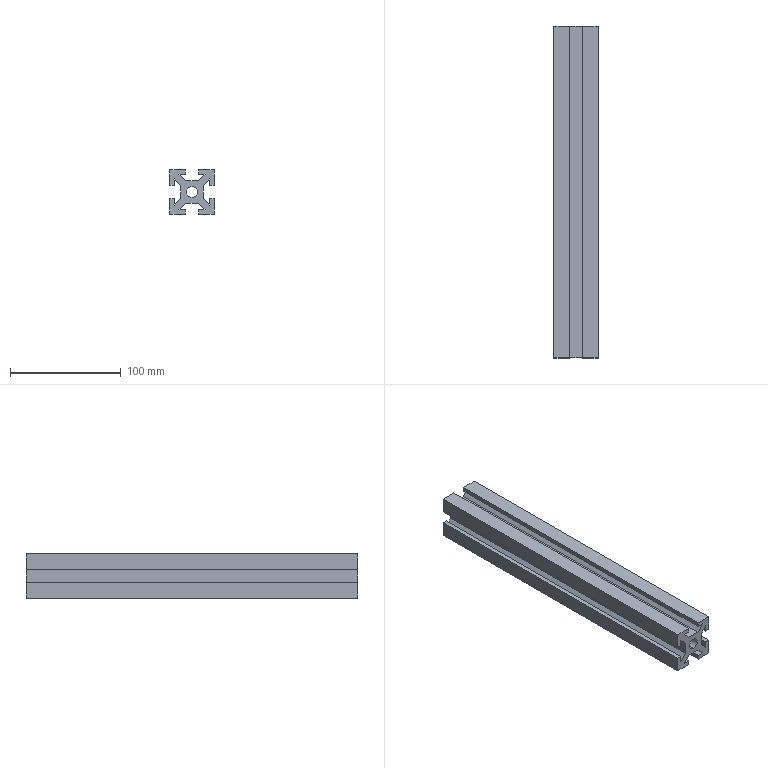Part | SolidWorks | features Extrusion 1 | 1 solid | 40 faces | box 40 x 300 x 40 mm | volume 272732 mm3 | plane 38 | cylinder 2 | commonest cylinder face diameters 10 x2
STEP:
#1=CARTESIAN_POINT('',(0.,300.,-5.));
#2=VERTEX_POINT('',#1);
#3=CARTESIAN_POINT('',(0.,300.,5.));
#4=VERTEX_POINT('',#3);
#5=CARTESIAN_POINT('',(0.,300.,0.));
#6=DIRECTION('',(0.,1.,0.));
#7=DIRECTION('',(0.,0.,1.));
#8=AXIS2_PLACEMENT_3D('',#5,#6,#7);
#9=CIRCLE('',#8,5.);
#10=EDGE_CURVE('',#2,#4,#9,.T.);
#11=ORIENTED_EDGE('',*,*,#10,.T.);
#12=CARTESIAN_POINT('',(0.,0.,5.));
#13=VERTEX_POINT('',#12);
#14=CARTESIAN_POINT('',(0.,300.,5.));
#15=DIRECTION('',(0.,-1.,0.));
#16=VECTOR('',#15,1000.);
#17=LINE('',#14,#16);
#18=EDGE_CURVE('',#4,#13,#17,.T.);
#19=ORIENTED_EDGE('',*,*,#18,.T.);
#20=CARTESIAN_POINT('',(0.,0.,-5.));
#21=VERTEX_POINT('',#20);
#22=CARTESIAN_POINT('',(0.,0.,0.));
#23=DIRECTION('',(0.,1.,0.));
#24=DIRECTION('',(0.,0.,1.));
#25=AXIS2_PLACEMENT_3D('',#22,#23,#24);
#26=CIRCLE('',#25,5.);
#27=EDGE_CURVE('',#21,#13,#26,.T.);
#28=ORIENTED_EDGE('',*,*,#27,.F.);
#29=CARTESIAN_POINT('',(0.,300.,-5.));
#30=DIRECTION('',(0.,-1.,0.));
#31=VECTOR('',#30,1000.);
#32=LINE('',#29,#31);
#33=EDGE_CURVE('',#2,#21,#32,.T.);
#34=ORIENTED_EDGE('',*,*,#33,.F.);
#35=EDGE_LOOP('',(#11,#19,#28,#34));
#36=FACE_OUTER_BOUND('',#35,.T.);
#37=CARTESIAN_POINT('',(0.,300.,0.));
#38=DIRECTION('',(0.,-1.,0.));
#39=DIRECTION('',(0.,0.,-1.));
#40=AXIS2_PLACEMENT_3D('',#37,#38,#39);
#41=CYLINDRICAL_SURFACE('',#40,5.);
#42=ADVANCED_FACE('',(#36),#41,.F.);
#43=CARTESIAN_POINT('',(6.,300.,20.));
#44=VERTEX_POINT('',#43);
#45=CARTESIAN_POINT('',(20.,300.,20.));
#46=VERTEX_POINT('',#45);
#47=CARTESIAN_POINT('',(6.,300.,20.));
#48=DIRECTION('',(1.,0.,0.));
#49=VECTOR('',#48,1000.);
#50=LINE('',#47,#49);
#51=EDGE_CURVE('',#44,#46,#50,.T.);
#52=ORIENTED_EDGE('',*,*,#51,.T.);
#53=CARTESIAN_POINT('',(20.,300.,6.));
#54=VERTEX_POINT('',#53);
#55=CARTESIAN_POINT('',(20.,300.,6.));
#56=DIRECTION('',(0.,0.,-1.));
#57=VECTOR('',#56,1000.);
#58=LINE('',#55,#57);
#59=EDGE_CURVE('',#46,#54,#58,.T.);
#60=ORIENTED_EDGE('',*,*,#59,.T.);
#61=CARTESIAN_POINT('',(16.,300.,6.));
#62=VERTEX_POINT('',#61);
#63=CARTESIAN_POINT('',(16.,300.,6.));
#64=DIRECTION('',(-1.,0.,0.));
#65=VECTOR('',#64,1000.);
#66=LINE('',#63,#65);
#67=EDGE_CURVE('',#54,#62,#66,.T.);
#68=ORIENTED_EDGE('',*,*,#67,.T.);
#69=CARTESIAN_POINT('',(16.,300.,11.757));
#70=VERTEX_POINT('',#69);
#71=CARTESIAN_POINT('',(16.,300.,11.757));
#72=DIRECTION('',(0.,0.,1.));
#73=VECTOR('',#72,1000.);
#74=LINE('',#71,#73);
#75=EDGE_CURVE('',#62,#70,#74,.T.);
#76=ORIENTED_EDGE('',*,*,#75,.T.);
#77=CARTESIAN_POINT('',(10.,300.,5.757));
#78=VERTEX_POINT('',#77);
#79=CARTESIAN_POINT('',(10.,300.,5.757));
#80=DIRECTION('',(-0.7071,0.,-0.7071));
#81=VECTOR('',#80,1000.);
#82=LINE('',#79,#81);
#83=EDGE_CURVE('',#70,#78,#82,.T.);
#84=ORIENTED_EDGE('',*,*,#83,.T.);
#85=CARTESIAN_POINT('',(10.,300.,-5.757));
#86=VERTEX_POINT('',#85);
#87=CARTESIAN_POINT('',(10.,300.,5.757));
#88=DIRECTION('',(0.,0.,-1.));
#89=VECTOR('',#88,1000.);
#90=LINE('',#87,#89);
#91=EDGE_CURVE('',#78,#86,#90,.T.);
#92=ORIENTED_EDGE('',*,*,#91,.T.);
#93=CARTESIAN_POINT('',(16.,300.,-11.757));
#94=VERTEX_POINT('',#93);
#95=CARTESIAN_POINT('',(16.,300.,-11.757));
#96=DIRECTION('',(0.7071,0.,-0.7071));
#97=VECTOR('',#96,1000.);
#98=LINE('',#95,#97);
#99=EDGE_CURVE('',#86,#94,#98,.T.);
#100=ORIENTED_EDGE('',*,*,#99,.T.);
#101=CARTESIAN_POINT('',(16.,300.,-6.));
#102=VERTEX_POINT('',#101);
#103=CARTESIAN_POINT('',(16.,300.,-6.));
#104=DIRECTION('',(0.,0.,1.));
#105=VECTOR('',#104,1000.);
#106=LINE('',#103,#105);
#107=EDGE_CURVE('',#94,#102,#106,.T.);
#108=ORIENTED_EDGE('',*,*,#107,.T.);
#109=CARTESIAN_POINT('',(20.,300.,-6.));
#110=VERTEX_POINT('',#109);
#111=CARTESIAN_POINT('',(20.,300.,-6.));
#112=DIRECTION('',(1.,0.,0.));
#113=VECTOR('',#112,1000.);
#114=LINE('',#111,#113);
#115=EDGE_CURVE('',#102,#110,#114,.T.);
#116=ORIENTED_EDGE('',*,*,#115,.T.);
#117=CARTESIAN_POINT('',(20.,300.,-20.));
#118=VERTEX_POINT('',#117);
#119=CARTESIAN_POINT('',(20.,300.,-20.));
#120=DIRECTION('',(0.,0.,-1.));
#121=VECTOR('',#120,1000.);
#122=LINE('',#119,#121);
#123=EDGE_CURVE('',#110,#118,#122,.T.);
#124=ORIENTED_EDGE('',*,*,#123,.T.);
#125=CARTESIAN_POINT('',(6.,300.,-20.));
#126=VERTEX_POINT('',#125);
#127=CARTESIAN_POINT('',(6.,300.,-20.));
#128=DIRECTION('',(-1.,0.,0.));
#129=VECTOR('',#128,1000.);
#130=LINE('',#127,#129);
#131=EDGE_CURVE('',#118,#126,#130,.T.);
#132=ORIENTED_EDGE('',*,*,#131,.T.);
#133=CARTESIAN_POINT('',(6.,300.,-16.));
#134=VERTEX_POINT('',#133);
#135=CARTESIAN_POINT('',(6.,300.,-16.));
#136=DIRECTION('',(0.,0.,1.));
#137=VECTOR('',#136,1000.);
#138=LINE('',#135,#137);
#139=EDGE_CURVE('',#126,#134,#138,.T.);
#140=ORIENTED_EDGE('',*,*,#139,.T.);
#141=CARTESIAN_POINT('',(11.757,300.,-16.));
#142=VERTEX_POINT('',#141);
#143=CARTESIAN_POINT('',(11.757,300.,-16.));
#144=DIRECTION('',(1.,0.,0.));
#145=VECTOR('',#144,1000.);
#146=LINE('',#143,#145);
#147=EDGE_CURVE('',#134,#142,#146,.T.);
#148=ORIENTED_EDGE('',*,*,#147,.T.);
#149=CARTESIAN_POINT('',(5.757,300.,-10.));
#150=VERTEX_POINT('',#149);
#151=CARTESIAN_POINT('',(5.757,300.,-10.));
#152=DIRECTION('',(-0.7071,0.,0.7071));
#153=VECTOR('',#152,1000.);
#154=LINE('',#151,#153);
#155=EDGE_CURVE('',#142,#150,#154,.T.);
#156=ORIENTED_EDGE('',*,*,#155,.T.);
#157=CARTESIAN_POINT('',(-5.757,300.,-10.));
#158=VERTEX_POINT('',#157);
#159=CARTESIAN_POINT('',(-5.757,300.,-10.));
#160=DIRECTION('',(-1.,0.,0.));
#161=VECTOR('',#160,1000.);
#162=LINE('',#159,#161);
#163=EDGE_CURVE('',#150,#158,#162,.T.);
#164=ORIENTED_EDGE('',*,*,#163,.T.);
#165=CARTESIAN_POINT('',(-11.757,300.,-16.));
#166=VERTEX_POINT('',#165);
#167=CARTESIAN_POINT('',(-11.757,300.,-16.));
#168=DIRECTION('',(-0.7071,0.,-0.7071));
#169=VECTOR('',#168,1000.);
#170=LINE('',#167,#169);
#171=EDGE_CURVE('',#158,#166,#170,.T.);
#172=ORIENTED_EDGE('',*,*,#171,.T.);
#173=CARTESIAN_POINT('',(-6.,300.,-16.));
#174=VERTEX_POINT('',#173);
#175=CARTESIAN_POINT('',(-6.,300.,-16.));
#176=DIRECTION('',(1.,0.,0.));
#177=VECTOR('',#176,1000.);
#178=LINE('',#175,#177);
#179=EDGE_CURVE('',#166,#174,#178,.T.);
#180=ORIENTED_EDGE('',*,*,#179,.T.);
#181=CARTESIAN_POINT('',(-6.,300.,-20.));
#182=VERTEX_POINT('',#181);
#183=CARTESIAN_POINT('',(-6.,300.,-20.));
#184=DIRECTION('',(0.,0.,-1.));
#185=VECTOR('',#184,1000.);
#186=LINE('',#183,#185);
#187=EDGE_CURVE('',#174,#182,#186,.T.);
#188=ORIENTED_EDGE('',*,*,#187,.T.);
#189=CARTESIAN_POINT('',(-20.,300.,-20.));
#190=VERTEX_POINT('',#189);
#191=CARTESIAN_POINT('',(-20.,300.,-20.));
#192=DIRECTION('',(-1.,0.,0.));
#193=VECTOR('',#192,1000.);
#194=LINE('',#191,#193);
#195=EDGE_CURVE('',#182,#190,#194,.T.);
#196=ORIENTED_EDGE('',*,*,#195,.T.);
#197=CARTESIAN_POINT('',(-20.,300.,-6.));
#198=VERTEX_POINT('',#197);
#199=CARTESIAN_POINT('',(-20.,300.,-20.));
#200=DIRECTION('',(0.,0.,1.));
#201=VECTOR('',#200,1000.);
#202=LINE('',#199,#201);
#203=EDGE_CURVE('',#190,#198,#202,.T.);
#204=ORIENTED_EDGE('',*,*,#203,.T.);
#205=CARTESIAN_POINT('',(-16.,300.,-6.));
#206=VERTEX_POINT('',#205);
#207=CARTESIAN_POINT('',(-16.,300.,-6.));
#208=DIRECTION('',(1.,0.,0.));
#209=VECTOR('',#208,1000.);
#210=LINE('',#207,#209);
#211=EDGE_CURVE('',#198,#206,#210,.T.);
#212=ORIENTED_EDGE('',*,*,#211,.T.);
#213=CARTESIAN_POINT('',(-16.,300.,-11.757));
#214=VERTEX_POINT('',#213);
#215=CARTESIAN_POINT('',(-16.,300.,-11.757));
#216=DIRECTION('',(0.,0.,-1.));
#217=VECTOR('',#216,1000.);
#218=LINE('',#215,#217);
#219=EDGE_CURVE('',#206,#214,#218,.T.);
#220=ORIENTED_EDGE('',*,*,#219,.T.);
#221=CARTESIAN_POINT('',(-10.,300.,-5.757));
#222=VERTEX_POINT('',#221);
#223=CARTESIAN_POINT('',(-10.,300.,-5.757));
#224=DIRECTION('',(0.7071,0.,0.7071));
#225=VECTOR('',#224,1000.);
#226=LINE('',#223,#225);
#227=EDGE_CURVE('',#214,#222,#226,.T.);
#228=ORIENTED_EDGE('',*,*,#227,.T.);
#229=CARTESIAN_POINT('',(-10.,300.,5.757));
#230=VERTEX_POINT('',#229);
#231=CARTESIAN_POINT('',(-10.,300.,5.757));
#232=DIRECTION('',(0.,0.,1.));
#233=VECTOR('',#232,1000.);
#234=LINE('',#231,#233);
#235=EDGE_CURVE('',#222,#230,#234,.T.);
#236=ORIENTED_EDGE('',*,*,#235,.T.);
#237=CARTESIAN_POINT('',(-16.,300.,11.757));
#238=VERTEX_POINT('',#237);
#239=CARTESIAN_POINT('',(-16.,300.,11.757));
#240=DIRECTION('',(-0.7071,0.,0.7071));
#241=VECTOR('',#240,1000.);
#242=LINE('',#239,#241);
#243=EDGE_CURVE('',#230,#238,#242,.T.);
#244=ORIENTED_EDGE('',*,*,#243,.T.);
#245=CARTESIAN_POINT('',(-16.,300.,6.));
#246=VERTEX_POINT('',#245);
#247=CARTESIAN_POINT('',(-16.,300.,6.));
#248=DIRECTION('',(0.,0.,-1.));
#249=VECTOR('',#248,1000.);
#250=LINE('',#247,#249);
#251=EDGE_CURVE('',#238,#246,#250,.T.);
#252=ORIENTED_EDGE('',*,*,#251,.T.);
#253=CARTESIAN_POINT('',(-20.,300.,6.));
#254=VERTEX_POINT('',#253);
#255=CARTESIAN_POINT('',(-20.,300.,6.));
#256=DIRECTION('',(-1.,0.,0.));
#257=VECTOR('',#256,1000.);
#258=LINE('',#255,#257);
#259=EDGE_CURVE('',#246,#254,#258,.T.);
#260=ORIENTED_EDGE('',*,*,#259,.T.);
#261=CARTESIAN_POINT('',(-20.,300.,20.));
#262=VERTEX_POINT('',#261);
#263=CARTESIAN_POINT('',(-20.,300.,6.));
#264=DIRECTION('',(0.,0.,1.));
#265=VECTOR('',#264,1000.);
#266=LINE('',#263,#265);
#267=EDGE_CURVE('',#254,#262,#266,.T.);
#268=ORIENTED_EDGE('',*,*,#267,.T.);
#269=CARTESIAN_POINT('',(-6.,300.,20.));
#270=VERTEX_POINT('',#269);
#271=CARTESIAN_POINT('',(-20.,300.,20.));
#272=DIRECTION('',(1.,0.,0.));
#273=VECTOR('',#272,1000.);
#274=LINE('',#271,#273);
#275=EDGE_CURVE('',#262,#270,#274,.T.);
#276=ORIENTED_EDGE('',*,*,#275,.T.);
#277=CARTESIAN_POINT('',(-6.,300.,16.));
#278=VERTEX_POINT('',#277);
#279=CARTESIAN_POINT('',(-6.,300.,16.));
#280=DIRECTION('',(0.,0.,-1.));
#281=VECTOR('',#280,1000.);
#282=LINE('',#279,#281);
#283=EDGE_CURVE('',#270,#278,#282,.T.);
#284=ORIENTED_EDGE('',*,*,#283,.T.);
#285=CARTESIAN_POINT('',(-11.757,300.,16.));
#286=VERTEX_POINT('',#285);
#287=CARTESIAN_POINT('',(-11.757,300.,16.));
#288=DIRECTION('',(-1.,0.,0.));
#289=VECTOR('',#288,1000.);
#290=LINE('',#287,#289);
#291=EDGE_CURVE('',#278,#286,#290,.T.);
#292=ORIENTED_EDGE('',*,*,#291,.T.);
#293=CARTESIAN_POINT('',(-5.757,300.,10.));
#294=VERTEX_POINT('',#293);
#295=CARTESIAN_POINT('',(-5.757,300.,10.));
#296=DIRECTION('',(0.7071,0.,-0.7071));
#297=VECTOR('',#296,1000.);
#298=LINE('',#295,#297);
#299=EDGE_CURVE('',#286,#294,#298,.T.);
#300=ORIENTED_EDGE('',*,*,#299,.T.);
#301=CARTESIAN_POINT('',(5.757,300.,10.));
#302=VERTEX_POINT('',#301);
#303=CARTESIAN_POINT('',(-5.757,300.,10.));
#304=DIRECTION('',(1.,0.,0.));
#305=VECTOR('',#304,1000.);
#306=LINE('',#303,#305);
#307=EDGE_CURVE('',#294,#302,#306,.T.);
#308=ORIENTED_EDGE('',*,*,#307,.T.);
#309=CARTESIAN_POINT('',(11.757,300.,16.));
#310=VERTEX_POINT('',#309);
#311=CARTESIAN_POINT('',(11.757,300.,16.));
#312=DIRECTION('',(0.7071,0.,0.7071));
#313=VECTOR('',#312,1000.);
#314=LINE('',#311,#313);
#315=EDGE_CURVE('',#302,#310,#314,.T.);
#316=ORIENTED_EDGE('',*,*,#315,.T.);
#317=CARTESIAN_POINT('',(6.,300.,16.));
#318=VERTEX_POINT('',#317);
#319=CARTESIAN_POINT('',(6.,300.,16.));
#320=DIRECTION('',(-1.,0.,0.));
#321=VECTOR('',#320,1000.);
#322=LINE('',#319,#321);
#323=EDGE_CURVE('',#310,#318,#322,.T.);
#324=ORIENTED_EDGE('',*,*,#323,.T.);
#325=CARTESIAN_POINT('',(6.,300.,20.));
#326=DIRECTION('',(0.,0.,1.));
#327=VECTOR('',#326,1000.);
#328=LINE('',#325,#327);
#329=EDGE_CURVE('',#318,#44,#328,.T.);
#330=ORIENTED_EDGE('',*,*,#329,.T.);
#331=EDGE_LOOP('',(#52,#60,#68,#76,#84,#92,#100,#108,#116,#124,#132,#140,#148,#156,#164,#172,#180,#188,#196,#204,#212,#220,#228,#236,#244,#252,#260,#268,#276,#284,#292,#300,#308,#316,#324,#330));
#332=FACE_OUTER_BOUND('',#331,.T.);
#333=ORIENTED_EDGE('',*,*,#10,.F.);
#334=CARTESIAN_POINT('',(0.,300.,0.));
#335=DIRECTION('',(0.,1.,0.));
#336=DIRECTION('',(0.,0.,1.));
#337=AXIS2_PLACEMENT_3D('',#334,#335,#336);
#338=CIRCLE('',#337,5.);
#339=EDGE_CURVE('',#4,#2,#338,.T.);
#340=ORIENTED_EDGE('',*,*,#339,.F.);
#341=EDGE_LOOP('',(#333,#340));
#342=FACE_BOUND('',#341,.T.);
#343=CARTESIAN_POINT('',(0.,300.,0.));
#344=DIRECTION('',(0.,-1.,0.));
#345=DIRECTION('',(0.,0.,-1.));
#346=AXIS2_PLACEMENT_3D('',#343,#344,#345);
#347=PLANE('',#346);
#348=ADVANCED_FACE('',(#332,#342),#347,.F.);
#349=CARTESIAN_POINT('',(6.,0.,20.));
#350=VERTEX_POINT('',#349);
#351=CARTESIAN_POINT('',(20.,0.,20.));
#352=VERTEX_POINT('',#351);
#353=CARTESIAN_POINT('',(6.,0.,20.));
#354=DIRECTION('',(1.,0.,0.));
#355=VECTOR('',#354,1000.);
#356=LINE('',#353,#355);
#357=EDGE_CURVE('',#350,#352,#356,.T.);
#358=ORIENTED_EDGE('',*,*,#357,.F.);
#359=CARTESIAN_POINT('',(6.,0.,16.));
#360=VERTEX_POINT('',#359);
#361=CARTESIAN_POINT('',(6.,0.,20.));
#362=DIRECTION('',(0.,0.,1.));
#363=VECTOR('',#362,1000.);
#364=LINE('',#361,#363);
#365=EDGE_CURVE('',#360,#350,#364,.T.);
#366=ORIENTED_EDGE('',*,*,#365,.F.);
#367=CARTESIAN_POINT('',(11.757,0.,16.));
#368=VERTEX_POINT('',#367);
#369=CARTESIAN_POINT('',(6.,0.,16.));
#370=DIRECTION('',(-1.,0.,0.));
#371=VECTOR('',#370,1000.);
#372=LINE('',#369,#371);
#373=EDGE_CURVE('',#368,#360,#372,.T.);
#374=ORIENTED_EDGE('',*,*,#373,.F.);
#375=CARTESIAN_POINT('',(5.757,0.,10.));
#376=VERTEX_POINT('',#375);
#377=CARTESIAN_POINT('',(11.757,0.,16.));
#378=DIRECTION('',(0.7071,0.,0.7071));
#379=VECTOR('',#378,1000.);
#380=LINE('',#377,#379);
#381=EDGE_CURVE('',#376,#368,#380,.T.);
#382=ORIENTED_EDGE('',*,*,#381,.F.);
#383=CARTESIAN_POINT('',(-5.757,0.,10.));
#384=VERTEX_POINT('',#383);
#385=CARTESIAN_POINT('',(-5.757,0.,10.));
#386=DIRECTION('',(1.,0.,0.));
#387=VECTOR('',#386,1000.);
#388=LINE('',#385,#387);
#389=EDGE_CURVE('',#384,#376,#388,.T.);
#390=ORIENTED_EDGE('',*,*,#389,.F.);
#391=CARTESIAN_POINT('',(-11.757,0.,16.));
#392=VERTEX_POINT('',#391);
#393=CARTESIAN_POINT('',(-5.757,0.,10.));
#394=DIRECTION('',(0.7071,0.,-0.7071));
#395=VECTOR('',#394,1000.);
#396=LINE('',#393,#395);
#397=EDGE_CURVE('',#392,#384,#396,.T.);
#398=ORIENTED_EDGE('',*,*,#397,.F.);
#399=CARTESIAN_POINT('',(-6.,0.,16.));
#400=VERTEX_POINT('',#399);
#401=CARTESIAN_POINT('',(-11.757,0.,16.));
#402=DIRECTION('',(-1.,0.,0.));
#403=VECTOR('',#402,1000.);
#404=LINE('',#401,#403);
#405=EDGE_CURVE('',#400,#392,#404,.T.);
#406=ORIENTED_EDGE('',*,*,#405,.F.);
#407=CARTESIAN_POINT('',(-6.,0.,20.));
#408=VERTEX_POINT('',#407);
#409=CARTESIAN_POINT('',(-6.,0.,16.));
#410=DIRECTION('',(0.,0.,-1.));
#411=VECTOR('',#410,1000.);
#412=LINE('',#409,#411);
#413=EDGE_CURVE('',#408,#400,#412,.T.);
#414=ORIENTED_EDGE('',*,*,#413,.F.);
#415=CARTESIAN_POINT('',(-20.,0.,20.));
#416=VERTEX_POINT('',#415);
#417=CARTESIAN_POINT('',(-20.,0.,20.));
#418=DIRECTION('',(1.,0.,0.));
#419=VECTOR('',#418,1000.);
#420=LINE('',#417,#419);
#421=EDGE_CURVE('',#416,#408,#420,.T.);
#422=ORIENTED_EDGE('',*,*,#421,.F.);
#423=CARTESIAN_POINT('',(-20.,0.,6.));
#424=VERTEX_POINT('',#423);
#425=CARTESIAN_POINT('',(-20.,0.,6.));
#426=DIRECTION('',(0.,0.,1.));
#427=VECTOR('',#426,1000.);
#428=LINE('',#425,#427);
#429=EDGE_CURVE('',#424,#416,#428,.T.);
#430=ORIENTED_EDGE('',*,*,#429,.F.);
#431=CARTESIAN_POINT('',(-16.,0.,6.));
#432=VERTEX_POINT('',#431);
#433=CARTESIAN_POINT('',(-20.,0.,6.));
#434=DIRECTION('',(-1.,0.,0.));
#435=VECTOR('',#434,1000.);
#436=LINE('',#433,#435);
#437=EDGE_CURVE('',#432,#424,#436,.T.);
#438=ORIENTED_EDGE('',*,*,#437,.F.);
#439=CARTESIAN_POINT('',(-16.,0.,11.757));
#440=VERTEX_POINT('',#439);
#441=CARTESIAN_POINT('',(-16.,0.,6.));
#442=DIRECTION('',(0.,0.,-1.));
#443=VECTOR('',#442,1000.);
#444=LINE('',#441,#443);
#445=EDGE_CURVE('',#440,#432,#444,.T.);
#446=ORIENTED_EDGE('',*,*,#445,.F.);
#447=CARTESIAN_POINT('',(-10.,0.,5.757));
#448=VERTEX_POINT('',#447);
#449=CARTESIAN_POINT('',(-16.,0.,11.757));
#450=DIRECTION('',(-0.7071,0.,0.7071));
#451=VECTOR('',#450,1000.);
#452=LINE('',#449,#451);
#453=EDGE_CURVE('',#448,#440,#452,.T.);
#454=ORIENTED_EDGE('',*,*,#453,.F.);
#455=CARTESIAN_POINT('',(-10.,0.,-5.757));
#456=VERTEX_POINT('',#455);
#457=CARTESIAN_POINT('',(-10.,0.,5.757));
#458=DIRECTION('',(0.,0.,1.));
#459=VECTOR('',#458,1000.);
#460=LINE('',#457,#459);
#461=EDGE_CURVE('',#456,#448,#460,.T.);
#462=ORIENTED_EDGE('',*,*,#461,.F.);
#463=CARTESIAN_POINT('',(-16.,0.,-11.757));
#464=VERTEX_POINT('',#463);
#465=CARTESIAN_POINT('',(-10.,0.,-5.757));
#466=DIRECTION('',(0.7071,0.,0.7071));
#467=VECTOR('',#466,1000.);
#468=LINE('',#465,#467);
#469=EDGE_CURVE('',#464,#456,#468,.T.);
#470=ORIENTED_EDGE('',*,*,#469,.F.);
#471=CARTESIAN_POINT('',(-16.,0.,-6.));
#472=VERTEX_POINT('',#471);
#473=CARTESIAN_POINT('',(-16.,0.,-11.757));
#474=DIRECTION('',(0.,0.,-1.));
#475=VECTOR('',#474,1000.);
#476=LINE('',#473,#475);
#477=EDGE_CURVE('',#472,#464,#476,.T.);
#478=ORIENTED_EDGE('',*,*,#477,.F.);
#479=CARTESIAN_POINT('',(-20.,0.,-6.));
#480=VERTEX_POINT('',#479);
#481=CARTESIAN_POINT('',(-16.,0.,-6.));
#482=DIRECTION('',(1.,0.,0.));
#483=VECTOR('',#482,1000.);
#484=LINE('',#481,#483);
#485=EDGE_CURVE('',#480,#472,#484,.T.);
#486=ORIENTED_EDGE('',*,*,#485,.F.);
#487=CARTESIAN_POINT('',(-20.,0.,-20.));
#488=VERTEX_POINT('',#487);
#489=CARTESIAN_POINT('',(-20.,0.,-20.));
#490=DIRECTION('',(0.,0.,1.));
#491=VECTOR('',#490,1000.);
#492=LINE('',#489,#491);
#493=EDGE_CURVE('',#488,#480,#492,.T.);
#494=ORIENTED_EDGE('',*,*,#493,.F.);
#495=CARTESIAN_POINT('',(-6.,0.,-20.));
#496=VERTEX_POINT('',#495);
#497=CARTESIAN_POINT('',(-20.,0.,-20.));
#498=DIRECTION('',(-1.,0.,0.));
#499=VECTOR('',#498,1000.);
#500=LINE('',#497,#499);
#501=EDGE_CURVE('',#496,#488,#500,.T.);
#502=ORIENTED_EDGE('',*,*,#501,.F.);
#503=CARTESIAN_POINT('',(-6.,0.,-16.));
#504=VERTEX_POINT('',#503);
#505=CARTESIAN_POINT('',(-6.,0.,-20.));
#506=DIRECTION('',(0.,0.,-1.));
#507=VECTOR('',#506,1000.);
#508=LINE('',#505,#507);
#509=EDGE_CURVE('',#504,#496,#508,.T.);
#510=ORIENTED_EDGE('',*,*,#509,.F.);
#511=CARTESIAN_POINT('',(-11.757,0.,-16.));
#512=VERTEX_POINT('',#511);
#513=CARTESIAN_POINT('',(-6.,0.,-16.));
#514=DIRECTION('',(1.,0.,0.));
#515=VECTOR('',#514,1000.);
#516=LINE('',#513,#515);
#517=EDGE_CURVE('',#512,#504,#516,.T.);
#518=ORIENTED_EDGE('',*,*,#517,.F.);
#519=CARTESIAN_POINT('',(-5.757,0.,-10.));
#520=VERTEX_POINT('',#519);
#521=CARTESIAN_POINT('',(-11.757,0.,-16.));
#522=DIRECTION('',(-0.7071,0.,-0.7071));
#523=VECTOR('',#522,1000.);
#524=LINE('',#521,#523);
#525=EDGE_CURVE('',#520,#512,#524,.T.);
#526=ORIENTED_EDGE('',*,*,#525,.F.);
#527=CARTESIAN_POINT('',(5.757,0.,-10.));
#528=VERTEX_POINT('',#527);
#529=CARTESIAN_POINT('',(-5.757,0.,-10.));
#530=DIRECTION('',(-1.,0.,0.));
#531=VECTOR('',#530,1000.);
#532=LINE('',#529,#531);
#533=EDGE_CURVE('',#528,#520,#532,.T.);
#534=ORIENTED_EDGE('',*,*,#533,.F.);
#535=CARTESIAN_POINT('',(11.757,0.,-16.));
#536=VERTEX_POINT('',#535);
#537=CARTESIAN_POINT('',(5.757,0.,-10.));
#538=DIRECTION('',(-0.7071,0.,0.7071));
#539=VECTOR('',#538,1000.);
#540=LINE('',#537,#539);
#541=EDGE_CURVE('',#536,#528,#540,.T.);
#542=ORIENTED_EDGE('',*,*,#541,.F.);
#543=CARTESIAN_POINT('',(6.,0.,-16.));
#544=VERTEX_POINT('',#543);
#545=CARTESIAN_POINT('',(11.757,0.,-16.));
#546=DIRECTION('',(1.,0.,0.));
#547=VECTOR('',#546,1000.);
#548=LINE('',#545,#547);
#549=EDGE_CURVE('',#544,#536,#548,.T.);
#550=ORIENTED_EDGE('',*,*,#549,.F.);
#551=CARTESIAN_POINT('',(6.,0.,-20.));
#552=VERTEX_POINT('',#551);
#553=CARTESIAN_POINT('',(6.,0.,-16.));
#554=DIRECTION('',(0.,0.,1.));
#555=VECTOR('',#554,1000.);
#556=LINE('',#553,#555);
#557=EDGE_CURVE('',#552,#544,#556,.T.);
#558=ORIENTED_EDGE('',*,*,#557,.F.);
#559=CARTESIAN_POINT('',(20.,0.,-20.));
#560=VERTEX_POINT('',#559);
#561=CARTESIAN_POINT('',(6.,0.,-20.));
#562=DIRECTION('',(-1.,0.,0.));
#563=VECTOR('',#562,1000.);
#564=LINE('',#561,#563);
#565=EDGE_CURVE('',#560,#552,#564,.T.);
#566=ORIENTED_EDGE('',*,*,#565,.F.);
#567=CARTESIAN_POINT('',(20.,0.,-6.));
#568=VERTEX_POINT('',#567);
#569=CARTESIAN_POINT('',(20.,0.,-20.));
#570=DIRECTION('',(0.,0.,-1.));
#571=VECTOR('',#570,1000.);
#572=LINE('',#569,#571);
#573=EDGE_CURVE('',#568,#560,#572,.T.);
#574=ORIENTED_EDGE('',*,*,#573,.F.);
#575=CARTESIAN_POINT('',(16.,0.,-6.));
#576=VERTEX_POINT('',#575);
#577=CARTESIAN_POINT('',(20.,0.,-6.));
#578=DIRECTION('',(1.,0.,0.));
#579=VECTOR('',#578,1000.);
#580=LINE('',#577,#579);
#581=EDGE_CURVE('',#576,#568,#580,.T.);
#582=ORIENTED_EDGE('',*,*,#581,.F.);
#583=CARTESIAN_POINT('',(16.,0.,-11.757));
#584=VERTEX_POINT('',#583);
#585=CARTESIAN_POINT('',(16.,0.,-6.));
#586=DIRECTION('',(0.,0.,1.));
#587=VECTOR('',#586,1000.);
#588=LINE('',#585,#587);
#589=EDGE_CURVE('',#584,#576,#588,.T.);
#590=ORIENTED_EDGE('',*,*,#589,.F.);
#591=CARTESIAN_POINT('',(10.,0.,-5.757));
#592=VERTEX_POINT('',#591);
#593=CARTESIAN_POINT('',(16.,0.,-11.757));
#594=DIRECTION('',(0.7071,0.,-0.7071));
#595=VECTOR('',#594,1000.);
#596=LINE('',#593,#595);
#597=EDGE_CURVE('',#592,#584,#596,.T.);
#598=ORIENTED_EDGE('',*,*,#597,.F.);
#599=CARTESIAN_POINT('',(10.,0.,5.757));
#600=VERTEX_POINT('',#599);
#601=CARTESIAN_POINT('',(10.,0.,5.757));
#602=DIRECTION('',(0.,0.,-1.));
#603=VECTOR('',#602,1000.);
#604=LINE('',#601,#603);
#605=EDGE_CURVE('',#600,#592,#604,.T.);
#606=ORIENTED_EDGE('',*,*,#605,.F.);
#607=CARTESIAN_POINT('',(16.,0.,11.757));
#608=VERTEX_POINT('',#607);
#609=CARTESIAN_POINT('',(10.,0.,5.757));
#610=DIRECTION('',(-0.7071,0.,-0.7071));
#611=VECTOR('',#610,1000.);
#612=LINE('',#609,#611);
#613=EDGE_CURVE('',#608,#600,#612,.T.);
#614=ORIENTED_EDGE('',*,*,#613,.F.);
#615=CARTESIAN_POINT('',(16.,0.,6.));
#616=VERTEX_POINT('',#615);
#617=CARTESIAN_POINT('',(16.,0.,11.757));
#618=DIRECTION('',(0.,0.,1.));
#619=VECTOR('',#618,1000.);
#620=LINE('',#617,#619);
#621=EDGE_CURVE('',#616,#608,#620,.T.);
#622=ORIENTED_EDGE('',*,*,#621,.F.);
#623=CARTESIAN_POINT('',(20.,0.,6.));
#624=VERTEX_POINT('',#623);
#625=CARTESIAN_POINT('',(16.,0.,6.));
#626=DIRECTION('',(-1.,0.,0.));
#627=VECTOR('',#626,1000.);
#628=LINE('',#625,#627);
#629=EDGE_CURVE('',#624,#616,#628,.T.);
#630=ORIENTED_EDGE('',*,*,#629,.F.);
#631=CARTESIAN_POINT('',(20.,0.,6.));
#632=DIRECTION('',(0.,0.,-1.));
#633=VECTOR('',#632,1000.);
#634=LINE('',#631,#633);
#635=EDGE_CURVE('',#352,#624,#634,.T.);
#636=ORIENTED_EDGE('',*,*,#635,.F.);
#637=EDGE_LOOP('',(#358,#366,#374,#382,#390,#398,#406,#414,#422,#430,#438,#446,#454,#462,#470,#478,#486,#494,#502,#510,#518,#526,#534,#542,#550,#558,#566,#574,#582,#590,#598,#606,#614,#622,#630,#636));
#638=FACE_OUTER_BOUND('',#637,.T.);
#639=ORIENTED_EDGE('',*,*,#27,.T.);
#640=CARTESIAN_POINT('',(0.,0.,0.));
#641=DIRECTION('',(0.,1.,0.));
#642=DIRECTION('',(0.,0.,1.));
#643=AXIS2_PLACEMENT_3D('',#640,#641,#642);
#644=CIRCLE('',#643,5.);
#645=EDGE_CURVE('',#13,#21,#644,.T.);
#646=ORIENTED_EDGE('',*,*,#645,.T.);
#647=EDGE_LOOP('',(#639,#646));
#648=FACE_BOUND('',#647,.T.);
#649=CARTESIAN_POINT('',(0.,0.,0.));
#650=DIRECTION('',(0.,-1.,0.));
#651=DIRECTION('',(0.,0.,-1.));
#652=AXIS2_PLACEMENT_3D('',#649,#650,#651);
#653=PLANE('',#652);
#654=ADVANCED_FACE('',(#638,#648),#653,.T.);
#655=ORIENTED_EDGE('',*,*,#357,.T.);
#656=CARTESIAN_POINT('',(20.,300.,20.));
#657=DIRECTION('',(0.,-1.,0.));
#658=VECTOR('',#657,1000.);
#659=LINE('',#656,#658);
#660=EDGE_CURVE('',#46,#352,#659,.T.);
#661=ORIENTED_EDGE('',*,*,#660,.F.);
#662=ORIENTED_EDGE('',*,*,#51,.F.);
#663=CARTESIAN_POINT('',(6.,300.,20.));
#664=DIRECTION('',(0.,-1.,0.));
#665=VECTOR('',#664,1000.);
#666=LINE('',#663,#665);
#667=EDGE_CURVE('',#44,#350,#666,.T.);
#668=ORIENTED_EDGE('',*,*,#667,.T.);
#669=EDGE_LOOP('',(#655,#661,#662,#668));
#670=FACE_OUTER_BOUND('',#669,.T.);
#671=CARTESIAN_POINT('',(6.,300.,20.));
#672=DIRECTION('',(0.,0.,-1.));
#673=DIRECTION('',(-1.,0.,0.));
#674=AXIS2_PLACEMENT_3D('',#671,#672,#673);
#675=PLANE('',#674);
#676=ADVANCED_FACE('',(#670),#675,.F.);
#677=ORIENTED_EDGE('',*,*,#635,.T.);
#678=CARTESIAN_POINT('',(20.,300.,6.));
#679=DIRECTION('',(0.,-1.,0.));
#680=VECTOR('',#679,1000.);
#681=LINE('',#678,#680);
#682=EDGE_CURVE('',#54,#624,#681,.T.);
#683=ORIENTED_EDGE('',*,*,#682,.F.);
#684=ORIENTED_EDGE('',*,*,#59,.F.);
#685=ORIENTED_EDGE('',*,*,#660,.T.);
#686=EDGE_LOOP('',(#677,#683,#684,#685));
#687=FACE_OUTER_BOUND('',#686,.T.);
#688=CARTESIAN_POINT('',(20.,300.,6.));
#689=DIRECTION('',(-1.,0.,0.));
#690=DIRECTION('',(0.,0.,1.));
#691=AXIS2_PLACEMENT_3D('',#688,#689,#690);
#692=PLANE('',#691);
#693=ADVANCED_FACE('',(#687),#692,.F.);
#694=ORIENTED_EDGE('',*,*,#629,.T.);
#695=CARTESIAN_POINT('',(16.,300.,6.));
#696=DIRECTION('',(0.,-1.,0.));
#697=VECTOR('',#696,1000.);
#698=LINE('',#695,#697);
#699=EDGE_CURVE('',#62,#616,#698,.T.);
#700=ORIENTED_EDGE('',*,*,#699,.F.);
#701=ORIENTED_EDGE('',*,*,#67,.F.);
#702=ORIENTED_EDGE('',*,*,#682,.T.);
#703=EDGE_LOOP('',(#694,#700,#701,#702));
#704=FACE_OUTER_BOUND('',#703,.T.);
#705=CARTESIAN_POINT('',(16.,300.,6.));
#706=DIRECTION('',(0.,0.,1.));
#707=DIRECTION('',(1.,0.,0.));
#708=AXIS2_PLACEMENT_3D('',#705,#706,#707);
#709=PLANE('',#708);
#710=ADVANCED_FACE('',(#704),#709,.F.);
#711=ORIENTED_EDGE('',*,*,#621,.T.);
#712=CARTESIAN_POINT('',(16.,300.,11.757));
#713=DIRECTION('',(0.,-1.,0.));
#714=VECTOR('',#713,1000.);
#715=LINE('',#712,#714);
#716=EDGE_CURVE('',#70,#608,#715,.T.);
#717=ORIENTED_EDGE('',*,*,#716,.F.);
#718=ORIENTED_EDGE('',*,*,#75,.F.);
#719=ORIENTED_EDGE('',*,*,#699,.T.);
#720=EDGE_LOOP('',(#711,#717,#718,#719));
#721=FACE_OUTER_BOUND('',#720,.T.);
#722=CARTESIAN_POINT('',(16.,300.,11.757));
#723=DIRECTION('',(1.,0.,0.));
#724=DIRECTION('',(0.,0.,-1.));
#725=AXIS2_PLACEMENT_3D('',#722,#723,#724);
#726=PLANE('',#725);
#727=ADVANCED_FACE('',(#721),#726,.F.);
#728=ORIENTED_EDGE('',*,*,#613,.T.);
#729=CARTESIAN_POINT('',(10.,300.,5.757));
#730=DIRECTION('',(0.,-1.,0.));
#731=VECTOR('',#730,1000.);
#732=LINE('',#729,#731);
#733=EDGE_CURVE('',#78,#600,#732,.T.);
#734=ORIENTED_EDGE('',*,*,#733,.F.);
#735=ORIENTED_EDGE('',*,*,#83,.F.);
#736=ORIENTED_EDGE('',*,*,#716,.T.);
#737=EDGE_LOOP('',(#728,#734,#735,#736));
#738=FACE_OUTER_BOUND('',#737,.T.);
#739=CARTESIAN_POINT('',(10.,300.,5.757));
#740=DIRECTION('',(-0.7071,0.,0.7071));
#741=DIRECTION('',(0.7071,0.,0.7071));
#742=AXIS2_PLACEMENT_3D('',#739,#740,#741);
#743=PLANE('',#742);
#744=ADVANCED_FACE('',(#738),#743,.F.);
#745=ORIENTED_EDGE('',*,*,#605,.T.);
#746=CARTESIAN_POINT('',(10.,300.,-5.757));
#747=DIRECTION('',(0.,-1.,0.));
#748=VECTOR('',#747,1000.);
#749=LINE('',#746,#748);
#750=EDGE_CURVE('',#86,#592,#749,.T.);
#751=ORIENTED_EDGE('',*,*,#750,.F.);
#752=ORIENTED_EDGE('',*,*,#91,.F.);
#753=ORIENTED_EDGE('',*,*,#733,.T.);
#754=EDGE_LOOP('',(#745,#751,#752,#753));
#755=FACE_OUTER_BOUND('',#754,.T.);
#756=CARTESIAN_POINT('',(10.,300.,5.757));
#757=DIRECTION('',(-1.,0.,0.));
#758=DIRECTION('',(0.,0.,1.));
#759=AXIS2_PLACEMENT_3D('',#756,#757,#758);
#760=PLANE('',#759);
#761=ADVANCED_FACE('',(#755),#760,.F.);
#762=ORIENTED_EDGE('',*,*,#597,.T.);
#763=CARTESIAN_POINT('',(16.,300.,-11.757));
#764=DIRECTION('',(0.,-1.,0.));
#765=VECTOR('',#764,1000.);
#766=LINE('',#763,#765);
#767=EDGE_CURVE('',#94,#584,#766,.T.);
#768=ORIENTED_EDGE('',*,*,#767,.F.);
#769=ORIENTED_EDGE('',*,*,#99,.F.);
#770=ORIENTED_EDGE('',*,*,#750,.T.);
#771=EDGE_LOOP('',(#762,#768,#769,#770));
#772=FACE_OUTER_BOUND('',#771,.T.);
#773=CARTESIAN_POINT('',(16.,300.,-11.757));
#774=DIRECTION('',(-0.7071,0.,-0.7071));
#775=DIRECTION('',(-0.7071,0.,0.7071));
#776=AXIS2_PLACEMENT_3D('',#773,#774,#775);
#777=PLANE('',#776);
#778=ADVANCED_FACE('',(#772),#777,.F.);
#779=ORIENTED_EDGE('',*,*,#589,.T.);
#780=CARTESIAN_POINT('',(16.,300.,-6.));
#781=DIRECTION('',(0.,-1.,0.));
#782=VECTOR('',#781,1000.);
#783=LINE('',#780,#782);
#784=EDGE_CURVE('',#102,#576,#783,.T.);
#785=ORIENTED_EDGE('',*,*,#784,.F.);
#786=ORIENTED_EDGE('',*,*,#107,.F.);
#787=ORIENTED_EDGE('',*,*,#767,.T.);
#788=EDGE_LOOP('',(#779,#785,#786,#787));
#789=FACE_OUTER_BOUND('',#788,.T.);
#790=CARTESIAN_POINT('',(16.,300.,-6.));
#791=DIRECTION('',(1.,0.,0.));
#792=DIRECTION('',(0.,0.,-1.));
#793=AXIS2_PLACEMENT_3D('',#790,#791,#792);
#794=PLANE('',#793);
#795=ADVANCED_FACE('',(#789),#794,.F.);
#796=ORIENTED_EDGE('',*,*,#581,.T.);
#797=CARTESIAN_POINT('',(20.,300.,-6.));
#798=DIRECTION('',(0.,-1.,0.));
#799=VECTOR('',#798,1000.);
#800=LINE('',#797,#799);
#801=EDGE_CURVE('',#110,#568,#800,.T.);
#802=ORIENTED_EDGE('',*,*,#801,.F.);
#803=ORIENTED_EDGE('',*,*,#115,.F.);
#804=ORIENTED_EDGE('',*,*,#784,.T.);
#805=EDGE_LOOP('',(#796,#802,#803,#804));
#806=FACE_OUTER_BOUND('',#805,.T.);
#807=CARTESIAN_POINT('',(20.,300.,-6.));
#808=DIRECTION('',(0.,0.,-1.));
#809=DIRECTION('',(-1.,0.,0.));
#810=AXIS2_PLACEMENT_3D('',#807,#808,#809);
#811=PLANE('',#810);
#812=ADVANCED_FACE('',(#806),#811,.F.);
#813=ORIENTED_EDGE('',*,*,#573,.T.);
#814=CARTESIAN_POINT('',(20.,300.,-20.));
#815=DIRECTION('',(0.,-1.,0.));
#816=VECTOR('',#815,1000.);
#817=LINE('',#814,#816);
#818=EDGE_CURVE('',#118,#560,#817,.T.);
#819=ORIENTED_EDGE('',*,*,#818,.F.);
#820=ORIENTED_EDGE('',*,*,#123,.F.);
#821=ORIENTED_EDGE('',*,*,#801,.T.);
#822=EDGE_LOOP('',(#813,#819,#820,#821));
#823=FACE_OUTER_BOUND('',#822,.T.);
#824=CARTESIAN_POINT('',(20.,300.,-20.));
#825=DIRECTION('',(-1.,0.,0.));
#826=DIRECTION('',(0.,0.,1.));
#827=AXIS2_PLACEMENT_3D('',#824,#825,#826);
#828=PLANE('',#827);
#829=ADVANCED_FACE('',(#823),#828,.F.);
#830=ORIENTED_EDGE('',*,*,#565,.T.);
#831=CARTESIAN_POINT('',(6.,300.,-20.));
#832=DIRECTION('',(0.,-1.,0.));
#833=VECTOR('',#832,1000.);
#834=LINE('',#831,#833);
#835=EDGE_CURVE('',#126,#552,#834,.T.);
#836=ORIENTED_EDGE('',*,*,#835,.F.);
#837=ORIENTED_EDGE('',*,*,#131,.F.);
#838=ORIENTED_EDGE('',*,*,#818,.T.);
#839=EDGE_LOOP('',(#830,#836,#837,#838));
#840=FACE_OUTER_BOUND('',#839,.T.);
#841=CARTESIAN_POINT('',(6.,300.,-20.));
#842=DIRECTION('',(0.,0.,1.));
#843=DIRECTION('',(1.,0.,0.));
#844=AXIS2_PLACEMENT_3D('',#841,#842,#843);
#845=PLANE('',#844);
#846=ADVANCED_FACE('',(#840),#845,.F.);
#847=ORIENTED_EDGE('',*,*,#557,.T.);
#848=CARTESIAN_POINT('',(6.,300.,-16.));
#849=DIRECTION('',(0.,-1.,0.));
#850=VECTOR('',#849,1000.);
#851=LINE('',#848,#850);
#852=EDGE_CURVE('',#134,#544,#851,.T.);
#853=ORIENTED_EDGE('',*,*,#852,.F.);
#854=ORIENTED_EDGE('',*,*,#139,.F.);
#855=ORIENTED_EDGE('',*,*,#835,.T.);
#856=EDGE_LOOP('',(#847,#853,#854,#855));
#857=FACE_OUTER_BOUND('',#856,.T.);
#858=CARTESIAN_POINT('',(6.,300.,-16.));
#859=DIRECTION('',(1.,0.,0.));
#860=DIRECTION('',(0.,0.,-1.));
#861=AXIS2_PLACEMENT_3D('',#858,#859,#860);
#862=PLANE('',#861);
#863=ADVANCED_FACE('',(#857),#862,.F.);
#864=ORIENTED_EDGE('',*,*,#549,.T.);
#865=CARTESIAN_POINT('',(11.757,300.,-16.));
#866=DIRECTION('',(0.,-1.,0.));
#867=VECTOR('',#866,1000.);
#868=LINE('',#865,#867);
#869=EDGE_CURVE('',#142,#536,#868,.T.);
#870=ORIENTED_EDGE('',*,*,#869,.F.);
#871=ORIENTED_EDGE('',*,*,#147,.F.);
#872=ORIENTED_EDGE('',*,*,#852,.T.);
#873=EDGE_LOOP('',(#864,#870,#871,#872));
#874=FACE_OUTER_BOUND('',#873,.T.);
#875=CARTESIAN_POINT('',(11.757,300.,-16.));
#876=DIRECTION('',(0.,0.,-1.));
#877=DIRECTION('',(-1.,0.,0.));
#878=AXIS2_PLACEMENT_3D('',#875,#876,#877);
#879=PLANE('',#878);
#880=ADVANCED_FACE('',(#874),#879,.F.);
#881=ORIENTED_EDGE('',*,*,#541,.T.);
#882=CARTESIAN_POINT('',(5.757,300.,-10.));
#883=DIRECTION('',(0.,-1.,0.));
#884=VECTOR('',#883,1000.);
#885=LINE('',#882,#884);
#886=EDGE_CURVE('',#150,#528,#885,.T.);
#887=ORIENTED_EDGE('',*,*,#886,.F.);
#888=ORIENTED_EDGE('',*,*,#155,.F.);
#889=ORIENTED_EDGE('',*,*,#869,.T.);
#890=EDGE_LOOP('',(#881,#887,#888,#889));
#891=FACE_OUTER_BOUND('',#890,.T.);
#892=CARTESIAN_POINT('',(5.757,300.,-10.));
#893=DIRECTION('',(0.7071,0.,0.7071));
#894=DIRECTION('',(0.7071,0.,-0.7071));
#895=AXIS2_PLACEMENT_3D('',#892,#893,#894);
#896=PLANE('',#895);
#897=ADVANCED_FACE('',(#891),#896,.F.);
#898=ORIENTED_EDGE('',*,*,#533,.T.);
#899=CARTESIAN_POINT('',(-5.757,300.,-10.));
#900=DIRECTION('',(0.,-1.,0.));
#901=VECTOR('',#900,1000.);
#902=LINE('',#899,#901);
#903=EDGE_CURVE('',#158,#520,#902,.T.);
#904=ORIENTED_EDGE('',*,*,#903,.F.);
#905=ORIENTED_EDGE('',*,*,#163,.F.);
#906=ORIENTED_EDGE('',*,*,#886,.T.);
#907=EDGE_LOOP('',(#898,#904,#905,#906));
#908=FACE_OUTER_BOUND('',#907,.T.);
#909=CARTESIAN_POINT('',(-5.757,300.,-10.));
#910=DIRECTION('',(0.,0.,1.));
#911=DIRECTION('',(1.,0.,0.));
#912=AXIS2_PLACEMENT_3D('',#909,#910,#911);
#913=PLANE('',#912);
#914=ADVANCED_FACE('',(#908),#913,.F.);
#915=ORIENTED_EDGE('',*,*,#525,.T.);
#916=CARTESIAN_POINT('',(-11.757,300.,-16.));
#917=DIRECTION('',(0.,-1.,0.));
#918=VECTOR('',#917,1000.);
#919=LINE('',#916,#918);
#920=EDGE_CURVE('',#166,#512,#919,.T.);
#921=ORIENTED_EDGE('',*,*,#920,.F.);
#922=ORIENTED_EDGE('',*,*,#171,.F.);
#923=ORIENTED_EDGE('',*,*,#903,.T.);
#924=EDGE_LOOP('',(#915,#921,#922,#923));
#925=FACE_OUTER_BOUND('',#924,.T.);
#926=CARTESIAN_POINT('',(-11.757,300.,-16.));
#927=DIRECTION('',(-0.7071,0.,0.7071));
#928=DIRECTION('',(0.7071,0.,0.7071));
#929=AXIS2_PLACEMENT_3D('',#926,#927,#928);
#930=PLANE('',#929);
#931=ADVANCED_FACE('',(#925),#930,.F.);
#932=ORIENTED_EDGE('',*,*,#517,.T.);
#933=CARTESIAN_POINT('',(-6.,300.,-16.));
#934=DIRECTION('',(0.,-1.,0.));
#935=VECTOR('',#934,1000.);
#936=LINE('',#933,#935);
#937=EDGE_CURVE('',#174,#504,#936,.T.);
#938=ORIENTED_EDGE('',*,*,#937,.F.);
#939=ORIENTED_EDGE('',*,*,#179,.F.);
#940=ORIENTED_EDGE('',*,*,#920,.T.);
#941=EDGE_LOOP('',(#932,#938,#939,#940));
#942=FACE_OUTER_BOUND('',#941,.T.);
#943=CARTESIAN_POINT('',(-6.,300.,-16.));
#944=DIRECTION('',(0.,0.,-1.));
#945=DIRECTION('',(-1.,0.,0.));
#946=AXIS2_PLACEMENT_3D('',#943,#944,#945);
#947=PLANE('',#946);
#948=ADVANCED_FACE('',(#942),#947,.F.);
#949=ORIENTED_EDGE('',*,*,#509,.T.);
#950=CARTESIAN_POINT('',(-6.,300.,-20.));
#951=DIRECTION('',(0.,-1.,0.));
#952=VECTOR('',#951,1000.);
#953=LINE('',#950,#952);
#954=EDGE_CURVE('',#182,#496,#953,.T.);
#955=ORIENTED_EDGE('',*,*,#954,.F.);
#956=ORIENTED_EDGE('',*,*,#187,.F.);
#957=ORIENTED_EDGE('',*,*,#937,.T.);
#958=EDGE_LOOP('',(#949,#955,#956,#957));
#959=FACE_OUTER_BOUND('',#958,.T.);
#960=CARTESIAN_POINT('',(-6.,300.,-20.));
#961=DIRECTION('',(-1.,0.,0.));
#962=DIRECTION('',(0.,0.,1.));
#963=AXIS2_PLACEMENT_3D('',#960,#961,#962);
#964=PLANE('',#963);
#965=ADVANCED_FACE('',(#959),#964,.F.);
#966=ORIENTED_EDGE('',*,*,#501,.T.);
#967=CARTESIAN_POINT('',(-20.,300.,-20.));
#968=DIRECTION('',(0.,-1.,0.));
#969=VECTOR('',#968,1000.);
#970=LINE('',#967,#969);
#971=EDGE_CURVE('',#190,#488,#970,.T.);
#972=ORIENTED_EDGE('',*,*,#971,.F.);
#973=ORIENTED_EDGE('',*,*,#195,.F.);
#974=ORIENTED_EDGE('',*,*,#954,.T.);
#975=EDGE_LOOP('',(#966,#972,#973,#974));
#976=FACE_OUTER_BOUND('',#975,.T.);
#977=CARTESIAN_POINT('',(-20.,300.,-20.));
#978=DIRECTION('',(0.,0.,1.));
#979=DIRECTION('',(1.,0.,0.));
#980=AXIS2_PLACEMENT_3D('',#977,#978,#979);
#981=PLANE('',#980);
#982=ADVANCED_FACE('',(#976),#981,.F.);
#983=ORIENTED_EDGE('',*,*,#493,.T.);
#984=CARTESIAN_POINT('',(-20.,300.,-6.));
#985=DIRECTION('',(0.,-1.,0.));
#986=VECTOR('',#985,1000.);
#987=LINE('',#984,#986);
#988=EDGE_CURVE('',#198,#480,#987,.T.);
#989=ORIENTED_EDGE('',*,*,#988,.F.);
#990=ORIENTED_EDGE('',*,*,#203,.F.);
#991=ORIENTED_EDGE('',*,*,#971,.T.);
#992=EDGE_LOOP('',(#983,#989,#990,#991));
#993=FACE_OUTER_BOUND('',#992,.T.);
#994=CARTESIAN_POINT('',(-20.,300.,-20.));
#995=DIRECTION('',(1.,0.,0.));
#996=DIRECTION('',(0.,0.,-1.));
#997=AXIS2_PLACEMENT_3D('',#994,#995,#996);
#998=PLANE('',#997);
#999=ADVANCED_FACE('',(#993),#998,.F.);
#1000=ORIENTED_EDGE('',*,*,#485,.T.);
#1001=CARTESIAN_POINT('',(-16.,300.,-6.));
#1002=DIRECTION('',(0.,-1.,0.));
#1003=VECTOR('',#1002,1000.);
#1004=LINE('',#1001,#1003);
#1005=EDGE_CURVE('',#206,#472,#1004,.T.);
#1006=ORIENTED_EDGE('',*,*,#1005,.F.);
#1007=ORIENTED_EDGE('',*,*,#211,.F.);
#1008=ORIENTED_EDGE('',*,*,#988,.T.);
#1009=EDGE_LOOP('',(#1000,#1006,#1007,#1008));
#1010=FACE_OUTER_BOUND('',#1009,.T.);
#1011=CARTESIAN_POINT('',(-16.,300.,-6.));
#1012=DIRECTION('',(0.,0.,-1.));
#1013=DIRECTION('',(-1.,0.,0.));
#1014=AXIS2_PLACEMENT_3D('',#1011,#1012,#1013);
#1015=PLANE('',#1014);
#1016=ADVANCED_FACE('',(#1010),#1015,.F.);
#1017=ORIENTED_EDGE('',*,*,#477,.T.);
#1018=CARTESIAN_POINT('',(-16.,300.,-11.757));
#1019=DIRECTION('',(0.,-1.,0.));
#1020=VECTOR('',#1019,1000.);
#1021=LINE('',#1018,#1020);
#1022=EDGE_CURVE('',#214,#464,#1021,.T.);
#1023=ORIENTED_EDGE('',*,*,#1022,.F.);
#1024=ORIENTED_EDGE('',*,*,#219,.F.);
#1025=ORIENTED_EDGE('',*,*,#1005,.T.);
#1026=EDGE_LOOP('',(#1017,#1023,#1024,#1025));
#1027=FACE_OUTER_BOUND('',#1026,.T.);
#1028=CARTESIAN_POINT('',(-16.,300.,-11.757));
#1029=DIRECTION('',(-1.,0.,0.));
#1030=DIRECTION('',(0.,0.,1.));
#1031=AXIS2_PLACEMENT_3D('',#1028,#1029,#1030);
#1032=PLANE('',#1031);
#1033=ADVANCED_FACE('',(#1027),#1032,.F.);
#1034=ORIENTED_EDGE('',*,*,#469,.T.);
#1035=CARTESIAN_POINT('',(-10.,300.,-5.757));
#1036=DIRECTION('',(0.,-1.,0.));
#1037=VECTOR('',#1036,1000.);
#1038=LINE('',#1035,#1037);
#1039=EDGE_CURVE('',#222,#456,#1038,.T.);
#1040=ORIENTED_EDGE('',*,*,#1039,.F.);
#1041=ORIENTED_EDGE('',*,*,#227,.F.);
#1042=ORIENTED_EDGE('',*,*,#1022,.T.);
#1043=EDGE_LOOP('',(#1034,#1040,#1041,#1042));
#1044=FACE_OUTER_BOUND('',#1043,.T.);
#1045=CARTESIAN_POINT('',(-10.,300.,-5.757));
#1046=DIRECTION('',(0.7071,0.,-0.7071));
#1047=DIRECTION('',(-0.7071,0.,-0.7071));
#1048=AXIS2_PLACEMENT_3D('',#1045,#1046,#1047);
#1049=PLANE('',#1048);
#1050=ADVANCED_FACE('',(#1044),#1049,.F.);
#1051=ORIENTED_EDGE('',*,*,#461,.T.);
#1052=CARTESIAN_POINT('',(-10.,300.,5.757));
#1053=DIRECTION('',(0.,-1.,0.));
#1054=VECTOR('',#1053,1000.);
#1055=LINE('',#1052,#1054);
#1056=EDGE_CURVE('',#230,#448,#1055,.T.);
#1057=ORIENTED_EDGE('',*,*,#1056,.F.);
#1058=ORIENTED_EDGE('',*,*,#235,.F.);
#1059=ORIENTED_EDGE('',*,*,#1039,.T.);
#1060=EDGE_LOOP('',(#1051,#1057,#1058,#1059));
#1061=FACE_OUTER_BOUND('',#1060,.T.);
#1062=CARTESIAN_POINT('',(-10.,300.,5.757));
#1063=DIRECTION('',(1.,0.,0.));
#1064=DIRECTION('',(0.,0.,-1.));
#1065=AXIS2_PLACEMENT_3D('',#1062,#1063,#1064);
#1066=PLANE('',#1065);
#1067=ADVANCED_FACE('',(#1061),#1066,.F.);
#1068=ORIENTED_EDGE('',*,*,#453,.T.);
#1069=CARTESIAN_POINT('',(-16.,300.,11.757));
#1070=DIRECTION('',(0.,-1.,0.));
#1071=VECTOR('',#1070,1000.);
#1072=LINE('',#1069,#1071);
#1073=EDGE_CURVE('',#238,#440,#1072,.T.);
#1074=ORIENTED_EDGE('',*,*,#1073,.F.);
#1075=ORIENTED_EDGE('',*,*,#243,.F.);
#1076=ORIENTED_EDGE('',*,*,#1056,.T.);
#1077=EDGE_LOOP('',(#1068,#1074,#1075,#1076));
#1078=FACE_OUTER_BOUND('',#1077,.T.);
#1079=CARTESIAN_POINT('',(-16.,300.,11.757));
#1080=DIRECTION('',(0.7071,0.,0.7071));
#1081=DIRECTION('',(0.7071,0.,-0.7071));
#1082=AXIS2_PLACEMENT_3D('',#1079,#1080,#1081);
#1083=PLANE('',#1082);
#1084=ADVANCED_FACE('',(#1078),#1083,.F.);
#1085=ORIENTED_EDGE('',*,*,#445,.T.);
#1086=CARTESIAN_POINT('',(-16.,300.,6.));
#1087=DIRECTION('',(0.,-1.,0.));
#1088=VECTOR('',#1087,1000.);
#1089=LINE('',#1086,#1088);
#1090=EDGE_CURVE('',#246,#432,#1089,.T.);
#1091=ORIENTED_EDGE('',*,*,#1090,.F.);
#1092=ORIENTED_EDGE('',*,*,#251,.F.);
#1093=ORIENTED_EDGE('',*,*,#1073,.T.);
#1094=EDGE_LOOP('',(#1085,#1091,#1092,#1093));
#1095=FACE_OUTER_BOUND('',#1094,.T.);
#1096=CARTESIAN_POINT('',(-16.,300.,6.));
#1097=DIRECTION('',(-1.,0.,0.));
#1098=DIRECTION('',(0.,0.,1.));
#1099=AXIS2_PLACEMENT_3D('',#1096,#1097,#1098);
#1100=PLANE('',#1099);
#1101=ADVANCED_FACE('',(#1095),#1100,.F.);
#1102=ORIENTED_EDGE('',*,*,#437,.T.);
#1103=CARTESIAN_POINT('',(-20.,300.,6.));
#1104=DIRECTION('',(0.,-1.,0.));
#1105=VECTOR('',#1104,1000.);
#1106=LINE('',#1103,#1105);
#1107=EDGE_CURVE('',#254,#424,#1106,.T.);
#1108=ORIENTED_EDGE('',*,*,#1107,.F.);
#1109=ORIENTED_EDGE('',*,*,#259,.F.);
#1110=ORIENTED_EDGE('',*,*,#1090,.T.);
#1111=EDGE_LOOP('',(#1102,#1108,#1109,#1110));
#1112=FACE_OUTER_BOUND('',#1111,.T.);
#1113=CARTESIAN_POINT('',(-20.,300.,6.));
#1114=DIRECTION('',(0.,0.,1.));
#1115=DIRECTION('',(1.,0.,0.));
#1116=AXIS2_PLACEMENT_3D('',#1113,#1114,#1115);
#1117=PLANE('',#1116);
#1118=ADVANCED_FACE('',(#1112),#1117,.F.);
#1119=ORIENTED_EDGE('',*,*,#429,.T.);
#1120=CARTESIAN_POINT('',(-20.,300.,20.));
#1121=DIRECTION('',(0.,-1.,0.));
#1122=VECTOR('',#1121,1000.);
#1123=LINE('',#1120,#1122);
#1124=EDGE_CURVE('',#262,#416,#1123,.T.);
#1125=ORIENTED_EDGE('',*,*,#1124,.F.);
#1126=ORIENTED_EDGE('',*,*,#267,.F.);
#1127=ORIENTED_EDGE('',*,*,#1107,.T.);
#1128=EDGE_LOOP('',(#1119,#1125,#1126,#1127));
#1129=FACE_OUTER_BOUND('',#1128,.T.);
#1130=CARTESIAN_POINT('',(-20.,300.,6.));
#1131=DIRECTION('',(1.,0.,0.));
#1132=DIRECTION('',(0.,0.,-1.));
#1133=AXIS2_PLACEMENT_3D('',#1130,#1131,#1132);
#1134=PLANE('',#1133);
#1135=ADVANCED_FACE('',(#1129),#1134,.F.);
#1136=ORIENTED_EDGE('',*,*,#421,.T.);
#1137=CARTESIAN_POINT('',(-6.,300.,20.));
#1138=DIRECTION('',(0.,-1.,0.));
#1139=VECTOR('',#1138,1000.);
#1140=LINE('',#1137,#1139);
#1141=EDGE_CURVE('',#270,#408,#1140,.T.);
#1142=ORIENTED_EDGE('',*,*,#1141,.F.);
#1143=ORIENTED_EDGE('',*,*,#275,.F.);
#1144=ORIENTED_EDGE('',*,*,#1124,.T.);
#1145=EDGE_LOOP('',(#1136,#1142,#1143,#1144));
#1146=FACE_OUTER_BOUND('',#1145,.T.);
#1147=CARTESIAN_POINT('',(-20.,300.,20.));
#1148=DIRECTION('',(0.,0.,-1.));
#1149=DIRECTION('',(-1.,0.,0.));
#1150=AXIS2_PLACEMENT_3D('',#1147,#1148,#1149);
#1151=PLANE('',#1150);
#1152=ADVANCED_FACE('',(#1146),#1151,.F.);
#1153=ORIENTED_EDGE('',*,*,#413,.T.);
#1154=CARTESIAN_POINT('',(-6.,300.,16.));
#1155=DIRECTION('',(0.,-1.,0.));
#1156=VECTOR('',#1155,1000.);
#1157=LINE('',#1154,#1156);
#1158=EDGE_CURVE('',#278,#400,#1157,.T.);
#1159=ORIENTED_EDGE('',*,*,#1158,.F.);
#1160=ORIENTED_EDGE('',*,*,#283,.F.);
#1161=ORIENTED_EDGE('',*,*,#1141,.T.);
#1162=EDGE_LOOP('',(#1153,#1159,#1160,#1161));
#1163=FACE_OUTER_BOUND('',#1162,.T.);
#1164=CARTESIAN_POINT('',(-6.,300.,16.));
#1165=DIRECTION('',(-1.,0.,0.));
#1166=DIRECTION('',(0.,0.,1.));
#1167=AXIS2_PLACEMENT_3D('',#1164,#1165,#1166);
#1168=PLANE('',#1167);
#1169=ADVANCED_FACE('',(#1163),#1168,.F.);
#1170=ORIENTED_EDGE('',*,*,#405,.T.);
#1171=CARTESIAN_POINT('',(-11.757,300.,16.));
#1172=DIRECTION('',(0.,-1.,0.));
#1173=VECTOR('',#1172,1000.);
#1174=LINE('',#1171,#1173);
#1175=EDGE_CURVE('',#286,#392,#1174,.T.);
#1176=ORIENTED_EDGE('',*,*,#1175,.F.);
#1177=ORIENTED_EDGE('',*,*,#291,.F.);
#1178=ORIENTED_EDGE('',*,*,#1158,.T.);
#1179=EDGE_LOOP('',(#1170,#1176,#1177,#1178));
#1180=FACE_OUTER_BOUND('',#1179,.T.);
#1181=CARTESIAN_POINT('',(-11.757,300.,16.));
#1182=DIRECTION('',(0.,0.,1.));
#1183=DIRECTION('',(1.,0.,0.));
#1184=AXIS2_PLACEMENT_3D('',#1181,#1182,#1183);
#1185=PLANE('',#1184);
#1186=ADVANCED_FACE('',(#1180),#1185,.F.);
#1187=ORIENTED_EDGE('',*,*,#397,.T.);
#1188=CARTESIAN_POINT('',(-5.757,300.,10.));
#1189=DIRECTION('',(0.,-1.,0.));
#1190=VECTOR('',#1189,1000.);
#1191=LINE('',#1188,#1190);
#1192=EDGE_CURVE('',#294,#384,#1191,.T.);
#1193=ORIENTED_EDGE('',*,*,#1192,.F.);
#1194=ORIENTED_EDGE('',*,*,#299,.F.);
#1195=ORIENTED_EDGE('',*,*,#1175,.T.);
#1196=EDGE_LOOP('',(#1187,#1193,#1194,#1195));
#1197=FACE_OUTER_BOUND('',#1196,.T.);
#1198=CARTESIAN_POINT('',(-5.757,300.,10.));
#1199=DIRECTION('',(-0.7071,0.,-0.7071));
#1200=DIRECTION('',(-0.7071,0.,0.7071));
#1201=AXIS2_PLACEMENT_3D('',#1198,#1199,#1200);
#1202=PLANE('',#1201);
#1203=ADVANCED_FACE('',(#1197),#1202,.F.);
#1204=ORIENTED_EDGE('',*,*,#389,.T.);
#1205=CARTESIAN_POINT('',(5.757,300.,10.));
#1206=DIRECTION('',(0.,-1.,0.));
#1207=VECTOR('',#1206,1000.);
#1208=LINE('',#1205,#1207);
#1209=EDGE_CURVE('',#302,#376,#1208,.T.);
#1210=ORIENTED_EDGE('',*,*,#1209,.F.);
#1211=ORIENTED_EDGE('',*,*,#307,.F.);
#1212=ORIENTED_EDGE('',*,*,#1192,.T.);
#1213=EDGE_LOOP('',(#1204,#1210,#1211,#1212));
#1214=FACE_OUTER_BOUND('',#1213,.T.);
#1215=CARTESIAN_POINT('',(-5.757,300.,10.));
#1216=DIRECTION('',(0.,0.,-1.));
#1217=DIRECTION('',(-1.,0.,0.));
#1218=AXIS2_PLACEMENT_3D('',#1215,#1216,#1217);
#1219=PLANE('',#1218);
#1220=ADVANCED_FACE('',(#1214),#1219,.F.);
#1221=ORIENTED_EDGE('',*,*,#381,.T.);
#1222=CARTESIAN_POINT('',(11.757,300.,16.));
#1223=DIRECTION('',(0.,-1.,0.));
#1224=VECTOR('',#1223,1000.);
#1225=LINE('',#1222,#1224);
#1226=EDGE_CURVE('',#310,#368,#1225,.T.);
#1227=ORIENTED_EDGE('',*,*,#1226,.F.);
#1228=ORIENTED_EDGE('',*,*,#315,.F.);
#1229=ORIENTED_EDGE('',*,*,#1209,.T.);
#1230=EDGE_LOOP('',(#1221,#1227,#1228,#1229));
#1231=FACE_OUTER_BOUND('',#1230,.T.);
#1232=CARTESIAN_POINT('',(11.757,300.,16.));
#1233=DIRECTION('',(0.7071,0.,-0.7071));
#1234=DIRECTION('',(-0.7071,0.,-0.7071));
#1235=AXIS2_PLACEMENT_3D('',#1232,#1233,#1234);
#1236=PLANE('',#1235);
#1237=ADVANCED_FACE('',(#1231),#1236,.F.);
#1238=ORIENTED_EDGE('',*,*,#373,.T.);
#1239=CARTESIAN_POINT('',(6.,300.,16.));
#1240=DIRECTION('',(0.,-1.,0.));
#1241=VECTOR('',#1240,1000.);
#1242=LINE('',#1239,#1241);
#1243=EDGE_CURVE('',#318,#360,#1242,.T.);
#1244=ORIENTED_EDGE('',*,*,#1243,.F.);
#1245=ORIENTED_EDGE('',*,*,#323,.F.);
#1246=ORIENTED_EDGE('',*,*,#1226,.T.);
#1247=EDGE_LOOP('',(#1238,#1244,#1245,#1246));
#1248=FACE_OUTER_BOUND('',#1247,.T.);
#1249=CARTESIAN_POINT('',(6.,300.,16.));
#1250=DIRECTION('',(0.,0.,1.));
#1251=DIRECTION('',(1.,0.,0.));
#1252=AXIS2_PLACEMENT_3D('',#1249,#1250,#1251);
#1253=PLANE('',#1252);
#1254=ADVANCED_FACE('',(#1248),#1253,.F.);
#1255=ORIENTED_EDGE('',*,*,#365,.T.);
#1256=ORIENTED_EDGE('',*,*,#667,.F.);
#1257=ORIENTED_EDGE('',*,*,#329,.F.);
#1258=ORIENTED_EDGE('',*,*,#1243,.T.);
#1259=EDGE_LOOP('',(#1255,#1256,#1257,#1258));
#1260=FACE_OUTER_BOUND('',#1259,.T.);
#1261=CARTESIAN_POINT('',(6.,300.,20.));
#1262=DIRECTION('',(1.,0.,0.));
#1263=DIRECTION('',(0.,0.,-1.));
#1264=AXIS2_PLACEMENT_3D('',#1261,#1262,#1263);
#1265=PLANE('',#1264);
#1266=ADVANCED_FACE('',(#1260),#1265,.F.);
#1267=ORIENTED_EDGE('',*,*,#18,.F.);
#1268=ORIENTED_EDGE('',*,*,#339,.T.);
#1269=ORIENTED_EDGE('',*,*,#33,.T.);
#1270=ORIENTED_EDGE('',*,*,#645,.F.);
#1271=EDGE_LOOP('',(#1267,#1268,#1269,#1270));
#1272=FACE_OUTER_BOUND('',#1271,.T.);
#1273=CARTESIAN_POINT('',(0.,300.,0.));
#1274=DIRECTION('',(0.,-1.,0.));
#1275=DIRECTION('',(0.,0.,-1.));
#1276=AXIS2_PLACEMENT_3D('',#1273,#1274,#1275);
#1277=CYLINDRICAL_SURFACE('',#1276,5.);
#1278=ADVANCED_FACE('',(#1272),#1277,.F.);
#1279=CLOSED_SHELL('',(#42,#348,#654,#676,#693,#710,#727,#744,#761,#778,#795,#812,#829,#846,#863,#880,#897,#914,#931,#948,#965,#982,#999,#1016,#1033,#1050,#1067,#1084,#1101,#1118,#1135,#1152,#1169,#1186,#1203,#1220,#1237,#1254,#1266,#1278));
#1280=MANIFOLD_SOLID_BREP('',#1279);
#1281=CARTESIAN_POINT('',(0.,0.,0.));
#1282=DIRECTION('',(0.,0.,1.));
#1283=DIRECTION('',(1.,0.,0.));
#1284=AXIS2_PLACEMENT_3D('',#1281,#1282,#1283);
#1285=(LENGTH_UNIT()NAMED_UNIT(*)SI_UNIT(.MILLI.,.METRE.));
#1286=UNCERTAINTY_MEASURE_WITH_UNIT(LENGTH_MEASURE(0.00001),#1285,'','');
#1287=(NAMED_UNIT(*)PLANE_ANGLE_UNIT()SI_UNIT($,.RADIAN.));
#1288=(NAMED_UNIT(*)SI_UNIT($,.STERADIAN.)SOLID_ANGLE_UNIT());
#1289=(GEOMETRIC_REPRESENTATION_CONTEXT(3)GLOBAL_UNCERTAINTY_ASSIGNED_CONTEXT((#1286))GLOBAL_UNIT_ASSIGNED_CONTEXT((#1285,#1287,#1288))REPRESENTATION_CONTEXT('',''));
#1290=ADVANCED_BREP_SHAPE_REPRESENTATION('',(#1280,#1284),#1289);